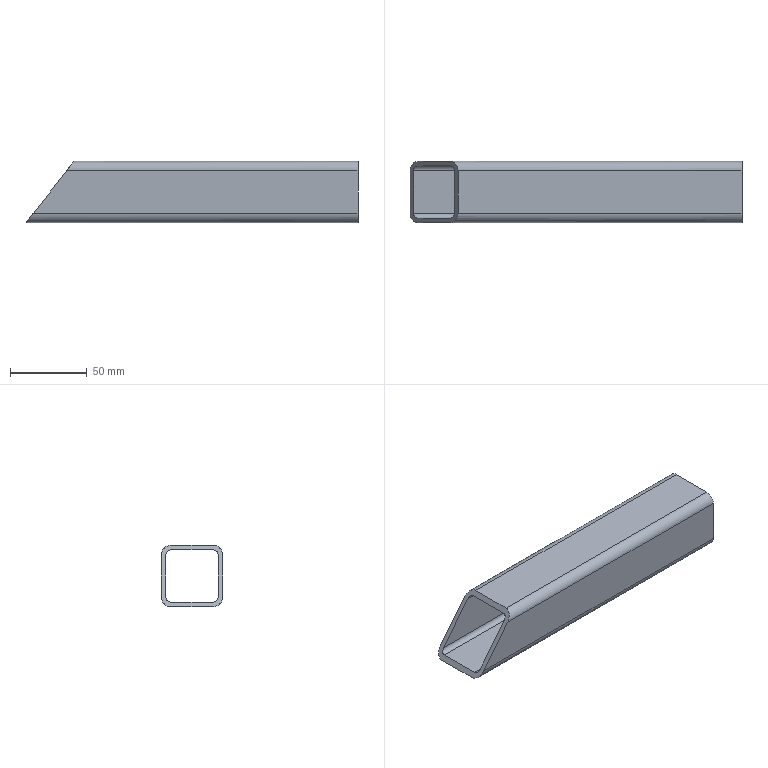Part | STEP file | SOLID | 1 solid | 18 faces | box 216.705 x 40 x 40 mm | volume 84594 mm3 | plane 10 | cylinder 8 | commonest cylinder face diameters 6 x4 12 x4